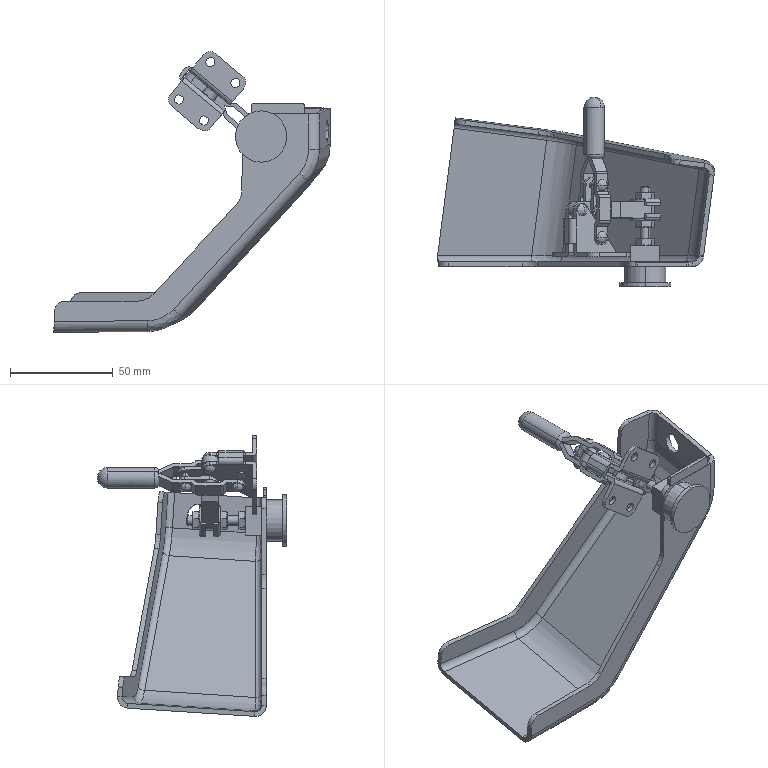Part | SolidWorks | 7 solids | 400 faces | box 134.657 x 92.265 x 136.571 mm | volume 37009 mm3 | plane 179 | cylinder 146 | cone 45 | sphere 18 | spline 6 | torus 6 | commonest cylinder face diameters 3 x26 10 x12 2 x10 7 x10 4 x9 4.4 x8